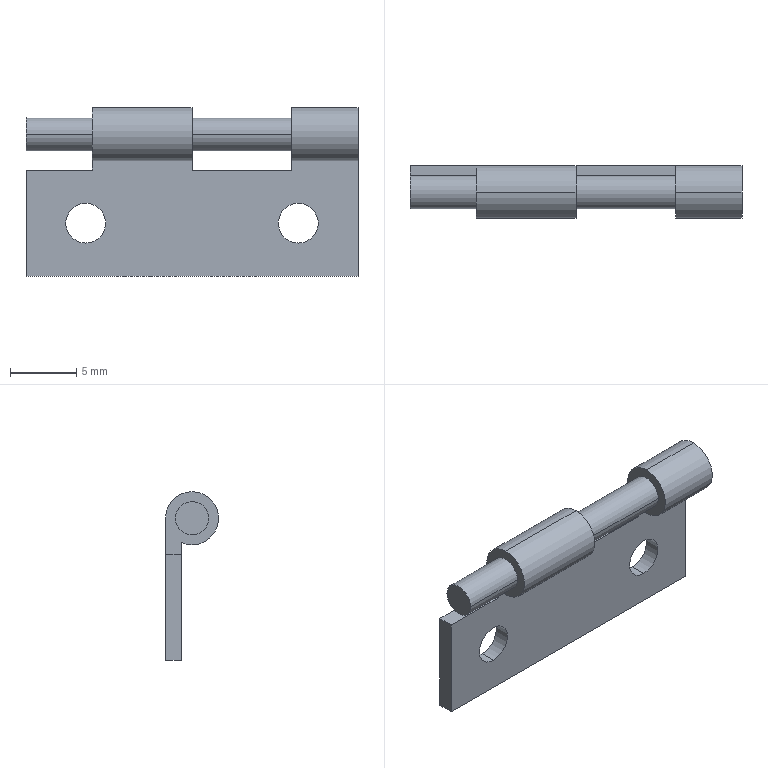Part | STEP file | 25 hinge-2 | 1 solid | 25 faces | box 25 x 4 x 12.7 mm | volume 462.157 mm3 | cylinder 14 | plane 11 | commonest cylinder face diameters 4 x6 2.5 x4 3 x4